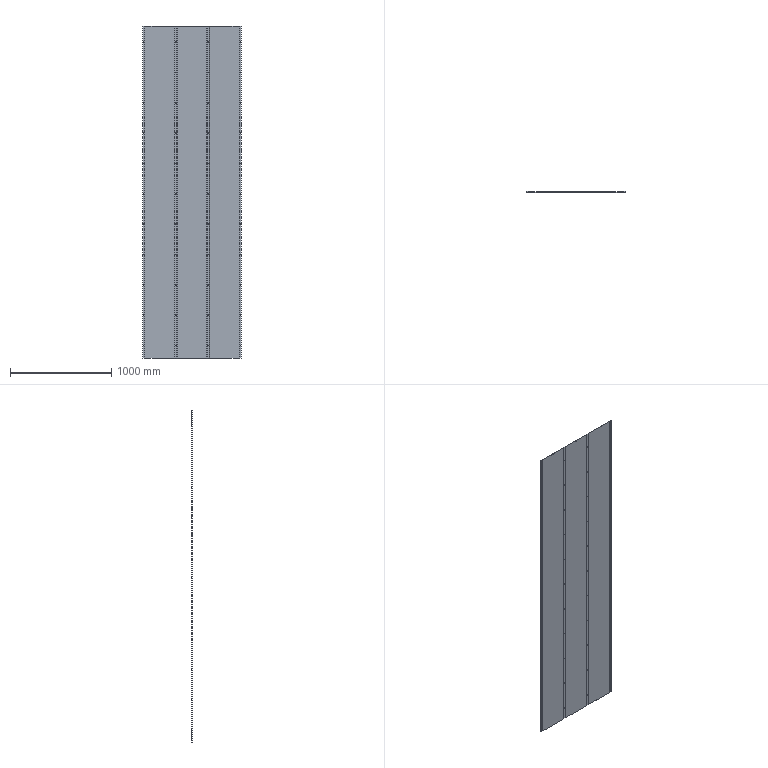Part | STEP file | SX-S18 | 1 solid | 196 faces | box 978 x 4.2 x 3283 mm | volume 3879324 mm3 | cylinder 115 | plane 81 | commonest cylinder face diameters 5.4 x88 0.4 x12 2.8 x12 10 x3